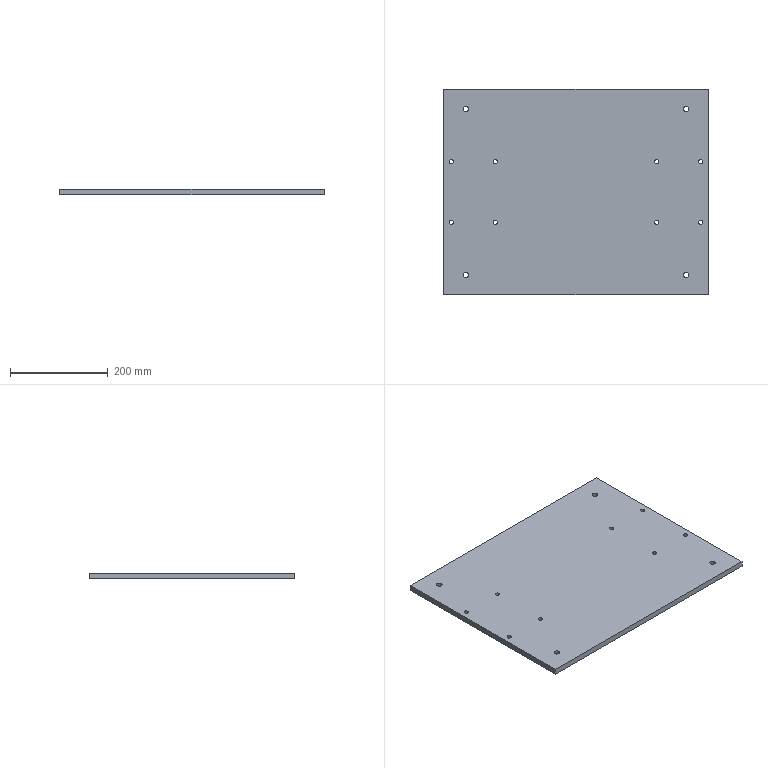Part | SolidWorks | features BaseBody 1 | 1 solid | 30 faces | box 540 x 420 x 12 mm | volume 2711591 mm3 | cylinder 24 | plane 6 | commonest cylinder face diameters 8.5 x16 11 x8
STEP:
#1=CARTESIAN_POINT('',(219.5,170.,-6.));
#2=VERTEX_POINT('',#1);
#3=CARTESIAN_POINT('',(230.5,170.,-6.));
#4=VERTEX_POINT('',#3);
#5=CARTESIAN_POINT('',(225.,170.,-6.));
#6=DIRECTION('',(0.,0.,1.));
#7=DIRECTION('',(1.,0.,0.));
#8=AXIS2_PLACEMENT_3D('',#5,#6,#7);
#9=CIRCLE('',#8,5.5);
#10=EDGE_CURVE('',#2,#4,#9,.T.);
#11=ORIENTED_EDGE('',*,*,#10,.F.);
#12=CARTESIAN_POINT('',(219.5,170.,6.));
#13=VERTEX_POINT('',#12);
#14=CARTESIAN_POINT('',(219.5,170.,-7.));
#15=DIRECTION('',(0.,0.,1.));
#16=VECTOR('',#15,1000.);
#17=LINE('',#14,#16);
#18=EDGE_CURVE('',#2,#13,#17,.T.);
#19=ORIENTED_EDGE('',*,*,#18,.T.);
#20=CARTESIAN_POINT('',(230.5,170.,6.));
#21=VERTEX_POINT('',#20);
#22=CARTESIAN_POINT('',(225.,170.,6.));
#23=DIRECTION('',(0.,0.,-1.));
#24=DIRECTION('',(1.,0.,0.));
#25=AXIS2_PLACEMENT_3D('',#22,#23,#24);
#26=CIRCLE('',#25,5.5);
#27=EDGE_CURVE('',#21,#13,#26,.T.);
#28=ORIENTED_EDGE('',*,*,#27,.F.);
#29=CARTESIAN_POINT('',(230.5,170.,-7.));
#30=DIRECTION('',(0.,0.,1.));
#31=VECTOR('',#30,1000.);
#32=LINE('',#29,#31);
#33=EDGE_CURVE('',#4,#21,#32,.T.);
#34=ORIENTED_EDGE('',*,*,#33,.F.);
#35=EDGE_LOOP('',(#11,#19,#28,#34));
#36=FACE_OUTER_BOUND('',#35,.T.);
#37=CARTESIAN_POINT('',(225.,170.,-7.));
#38=DIRECTION('',(0.,0.,1.));
#39=DIRECTION('',(1.,0.,0.));
#40=AXIS2_PLACEMENT_3D('',#37,#38,#39);
#41=CYLINDRICAL_SURFACE('',#40,5.5);
#42=ADVANCED_FACE('',(#36),#41,.F.);
#43=CARTESIAN_POINT('',(250.75,62.,-6.));
#44=VERTEX_POINT('',#43);
#45=CARTESIAN_POINT('',(259.25,62.,-6.));
#46=VERTEX_POINT('',#45);
#47=CARTESIAN_POINT('',(255.,62.,-6.));
#48=DIRECTION('',(0.,0.,1.));
#49=DIRECTION('',(1.,0.,0.));
#50=AXIS2_PLACEMENT_3D('',#47,#48,#49);
#51=CIRCLE('',#50,4.25);
#52=EDGE_CURVE('',#44,#46,#51,.T.);
#53=ORIENTED_EDGE('',*,*,#52,.F.);
#54=CARTESIAN_POINT('',(250.75,62.,6.));
#55=VERTEX_POINT('',#54);
#56=CARTESIAN_POINT('',(250.75,62.,-7.));
#57=DIRECTION('',(0.,0.,1.));
#58=VECTOR('',#57,1000.);
#59=LINE('',#56,#58);
#60=EDGE_CURVE('',#44,#55,#59,.T.);
#61=ORIENTED_EDGE('',*,*,#60,.T.);
#62=CARTESIAN_POINT('',(259.25,62.,6.));
#63=VERTEX_POINT('',#62);
#64=CARTESIAN_POINT('',(255.,62.,6.));
#65=DIRECTION('',(0.,0.,-1.));
#66=DIRECTION('',(1.,0.,0.));
#67=AXIS2_PLACEMENT_3D('',#64,#65,#66);
#68=CIRCLE('',#67,4.25);
#69=EDGE_CURVE('',#63,#55,#68,.T.);
#70=ORIENTED_EDGE('',*,*,#69,.F.);
#71=CARTESIAN_POINT('',(259.25,62.,-7.));
#72=DIRECTION('',(0.,0.,1.));
#73=VECTOR('',#72,1000.);
#74=LINE('',#71,#73);
#75=EDGE_CURVE('',#46,#63,#74,.T.);
#76=ORIENTED_EDGE('',*,*,#75,.F.);
#77=EDGE_LOOP('',(#53,#61,#70,#76));
#78=FACE_OUTER_BOUND('',#77,.T.);
#79=CARTESIAN_POINT('',(255.,62.,-7.));
#80=DIRECTION('',(0.,0.,1.));
#81=DIRECTION('',(1.,0.,0.));
#82=AXIS2_PLACEMENT_3D('',#79,#80,#81);
#83=CYLINDRICAL_SURFACE('',#82,4.25);
#84=ADVANCED_FACE('',(#78),#83,.F.);
#85=CARTESIAN_POINT('',(160.75,62.,-6.));
#86=VERTEX_POINT('',#85);
#87=CARTESIAN_POINT('',(169.25,62.,-6.));
#88=VERTEX_POINT('',#87);
#89=CARTESIAN_POINT('',(165.,62.,-6.));
#90=DIRECTION('',(0.,0.,1.));
#91=DIRECTION('',(1.,0.,0.));
#92=AXIS2_PLACEMENT_3D('',#89,#90,#91);
#93=CIRCLE('',#92,4.25);
#94=EDGE_CURVE('',#86,#88,#93,.T.);
#95=ORIENTED_EDGE('',*,*,#94,.F.);
#96=CARTESIAN_POINT('',(160.75,62.,6.));
#97=VERTEX_POINT('',#96);
#98=CARTESIAN_POINT('',(160.75,62.,-7.));
#99=DIRECTION('',(0.,0.,1.));
#100=VECTOR('',#99,1000.);
#101=LINE('',#98,#100);
#102=EDGE_CURVE('',#86,#97,#101,.T.);
#103=ORIENTED_EDGE('',*,*,#102,.T.);
#104=CARTESIAN_POINT('',(169.25,62.,6.));
#105=VERTEX_POINT('',#104);
#106=CARTESIAN_POINT('',(165.,62.,6.));
#107=DIRECTION('',(0.,0.,-1.));
#108=DIRECTION('',(1.,0.,0.));
#109=AXIS2_PLACEMENT_3D('',#106,#107,#108);
#110=CIRCLE('',#109,4.25);
#111=EDGE_CURVE('',#105,#97,#110,.T.);
#112=ORIENTED_EDGE('',*,*,#111,.F.);
#113=CARTESIAN_POINT('',(169.25,62.,-7.));
#114=DIRECTION('',(0.,0.,1.));
#115=VECTOR('',#114,1000.);
#116=LINE('',#113,#115);
#117=EDGE_CURVE('',#88,#105,#116,.T.);
#118=ORIENTED_EDGE('',*,*,#117,.F.);
#119=EDGE_LOOP('',(#95,#103,#112,#118));
#120=FACE_OUTER_BOUND('',#119,.T.);
#121=CARTESIAN_POINT('',(165.,62.,-7.));
#122=DIRECTION('',(0.,0.,1.));
#123=DIRECTION('',(1.,0.,0.));
#124=AXIS2_PLACEMENT_3D('',#121,#122,#123);
#125=CYLINDRICAL_SURFACE('',#124,4.25);
#126=ADVANCED_FACE('',(#120),#125,.F.);
#127=CARTESIAN_POINT('',(-230.5,170.,-6.));
#128=VERTEX_POINT('',#127);
#129=CARTESIAN_POINT('',(-219.5,170.,-6.));
#130=VERTEX_POINT('',#129);
#131=CARTESIAN_POINT('',(-225.,170.,-6.));
#132=DIRECTION('',(0.,0.,1.));
#133=DIRECTION('',(1.,0.,0.));
#134=AXIS2_PLACEMENT_3D('',#131,#132,#133);
#135=CIRCLE('',#134,5.5);
#136=EDGE_CURVE('',#128,#130,#135,.T.);
#137=ORIENTED_EDGE('',*,*,#136,.F.);
#138=CARTESIAN_POINT('',(-230.5,170.,6.));
#139=VERTEX_POINT('',#138);
#140=CARTESIAN_POINT('',(-230.5,170.,-7.));
#141=DIRECTION('',(0.,0.,1.));
#142=VECTOR('',#141,1000.);
#143=LINE('',#140,#142);
#144=EDGE_CURVE('',#128,#139,#143,.T.);
#145=ORIENTED_EDGE('',*,*,#144,.T.);
#146=CARTESIAN_POINT('',(-219.5,170.,6.));
#147=VERTEX_POINT('',#146);
#148=CARTESIAN_POINT('',(-225.,170.,6.));
#149=DIRECTION('',(0.,0.,-1.));
#150=DIRECTION('',(1.,0.,0.));
#151=AXIS2_PLACEMENT_3D('',#148,#149,#150);
#152=CIRCLE('',#151,5.5);
#153=EDGE_CURVE('',#147,#139,#152,.T.);
#154=ORIENTED_EDGE('',*,*,#153,.F.);
#155=CARTESIAN_POINT('',(-219.5,170.,-7.));
#156=DIRECTION('',(0.,0.,1.));
#157=VECTOR('',#156,1000.);
#158=LINE('',#155,#157);
#159=EDGE_CURVE('',#130,#147,#158,.T.);
#160=ORIENTED_EDGE('',*,*,#159,.F.);
#161=EDGE_LOOP('',(#137,#145,#154,#160));
#162=FACE_OUTER_BOUND('',#161,.T.);
#163=CARTESIAN_POINT('',(-225.,170.,-7.));
#164=DIRECTION('',(0.,0.,1.));
#165=DIRECTION('',(1.,0.,0.));
#166=AXIS2_PLACEMENT_3D('',#163,#164,#165);
#167=CYLINDRICAL_SURFACE('',#166,5.5);
#168=ADVANCED_FACE('',(#162),#167,.F.);
#169=CARTESIAN_POINT('',(-169.25,62.,-6.));
#170=VERTEX_POINT('',#169);
#171=CARTESIAN_POINT('',(-160.75,62.,-6.));
#172=VERTEX_POINT('',#171);
#173=CARTESIAN_POINT('',(-165.,62.,-6.));
#174=DIRECTION('',(0.,0.,1.));
#175=DIRECTION('',(1.,0.,0.));
#176=AXIS2_PLACEMENT_3D('',#173,#174,#175);
#177=CIRCLE('',#176,4.25);
#178=EDGE_CURVE('',#170,#172,#177,.T.);
#179=ORIENTED_EDGE('',*,*,#178,.F.);
#180=CARTESIAN_POINT('',(-169.25,62.,6.));
#181=VERTEX_POINT('',#180);
#182=CARTESIAN_POINT('',(-169.25,62.,-7.));
#183=DIRECTION('',(0.,0.,1.));
#184=VECTOR('',#183,1000.);
#185=LINE('',#182,#184);
#186=EDGE_CURVE('',#170,#181,#185,.T.);
#187=ORIENTED_EDGE('',*,*,#186,.T.);
#188=CARTESIAN_POINT('',(-160.75,62.,6.));
#189=VERTEX_POINT('',#188);
#190=CARTESIAN_POINT('',(-165.,62.,6.));
#191=DIRECTION('',(0.,0.,-1.));
#192=DIRECTION('',(1.,0.,0.));
#193=AXIS2_PLACEMENT_3D('',#190,#191,#192);
#194=CIRCLE('',#193,4.25);
#195=EDGE_CURVE('',#189,#181,#194,.T.);
#196=ORIENTED_EDGE('',*,*,#195,.F.);
#197=CARTESIAN_POINT('',(-160.75,62.,-7.));
#198=DIRECTION('',(0.,0.,1.));
#199=VECTOR('',#198,1000.);
#200=LINE('',#197,#199);
#201=EDGE_CURVE('',#172,#189,#200,.T.);
#202=ORIENTED_EDGE('',*,*,#201,.F.);
#203=EDGE_LOOP('',(#179,#187,#196,#202));
#204=FACE_OUTER_BOUND('',#203,.T.);
#205=CARTESIAN_POINT('',(-165.,62.,-7.));
#206=DIRECTION('',(0.,0.,1.));
#207=DIRECTION('',(1.,0.,0.));
#208=AXIS2_PLACEMENT_3D('',#205,#206,#207);
#209=CYLINDRICAL_SURFACE('',#208,4.25);
#210=ADVANCED_FACE('',(#204),#209,.F.);
#211=CARTESIAN_POINT('',(-259.25,62.,-6.));
#212=VERTEX_POINT('',#211);
#213=CARTESIAN_POINT('',(-250.75,62.,-6.));
#214=VERTEX_POINT('',#213);
#215=CARTESIAN_POINT('',(-255.,62.,-6.));
#216=DIRECTION('',(0.,0.,1.));
#217=DIRECTION('',(1.,0.,0.));
#218=AXIS2_PLACEMENT_3D('',#215,#216,#217);
#219=CIRCLE('',#218,4.25);
#220=EDGE_CURVE('',#212,#214,#219,.T.);
#221=ORIENTED_EDGE('',*,*,#220,.F.);
#222=CARTESIAN_POINT('',(-259.25,62.,6.));
#223=VERTEX_POINT('',#222);
#224=CARTESIAN_POINT('',(-259.25,62.,-7.));
#225=DIRECTION('',(0.,0.,1.));
#226=VECTOR('',#225,1000.);
#227=LINE('',#224,#226);
#228=EDGE_CURVE('',#212,#223,#227,.T.);
#229=ORIENTED_EDGE('',*,*,#228,.T.);
#230=CARTESIAN_POINT('',(-250.75,62.,6.));
#231=VERTEX_POINT('',#230);
#232=CARTESIAN_POINT('',(-255.,62.,6.));
#233=DIRECTION('',(0.,0.,-1.));
#234=DIRECTION('',(1.,0.,0.));
#235=AXIS2_PLACEMENT_3D('',#232,#233,#234);
#236=CIRCLE('',#235,4.25);
#237=EDGE_CURVE('',#231,#223,#236,.T.);
#238=ORIENTED_EDGE('',*,*,#237,.F.);
#239=CARTESIAN_POINT('',(-250.75,62.,-7.));
#240=DIRECTION('',(0.,0.,1.));
#241=VECTOR('',#240,1000.);
#242=LINE('',#239,#241);
#243=EDGE_CURVE('',#214,#231,#242,.T.);
#244=ORIENTED_EDGE('',*,*,#243,.F.);
#245=EDGE_LOOP('',(#221,#229,#238,#244));
#246=FACE_OUTER_BOUND('',#245,.T.);
#247=CARTESIAN_POINT('',(-255.,62.,-7.));
#248=DIRECTION('',(0.,0.,1.));
#249=DIRECTION('',(1.,0.,0.));
#250=AXIS2_PLACEMENT_3D('',#247,#248,#249);
#251=CYLINDRICAL_SURFACE('',#250,4.25);
#252=ADVANCED_FACE('',(#246),#251,.F.);
#253=CARTESIAN_POINT('',(250.75,-62.,-6.));
#254=VERTEX_POINT('',#253);
#255=CARTESIAN_POINT('',(259.25,-62.,-6.));
#256=VERTEX_POINT('',#255);
#257=CARTESIAN_POINT('',(255.,-62.,-6.));
#258=DIRECTION('',(0.,0.,1.));
#259=DIRECTION('',(1.,0.,0.));
#260=AXIS2_PLACEMENT_3D('',#257,#258,#259);
#261=CIRCLE('',#260,4.25);
#262=EDGE_CURVE('',#254,#256,#261,.T.);
#263=ORIENTED_EDGE('',*,*,#262,.F.);
#264=CARTESIAN_POINT('',(250.75,-62.,6.));
#265=VERTEX_POINT('',#264);
#266=CARTESIAN_POINT('',(250.75,-62.,-7.));
#267=DIRECTION('',(0.,0.,1.));
#268=VECTOR('',#267,1000.);
#269=LINE('',#266,#268);
#270=EDGE_CURVE('',#254,#265,#269,.T.);
#271=ORIENTED_EDGE('',*,*,#270,.T.);
#272=CARTESIAN_POINT('',(259.25,-62.,6.));
#273=VERTEX_POINT('',#272);
#274=CARTESIAN_POINT('',(255.,-62.,6.));
#275=DIRECTION('',(0.,0.,-1.));
#276=DIRECTION('',(1.,0.,0.));
#277=AXIS2_PLACEMENT_3D('',#274,#275,#276);
#278=CIRCLE('',#277,4.25);
#279=EDGE_CURVE('',#273,#265,#278,.T.);
#280=ORIENTED_EDGE('',*,*,#279,.F.);
#281=CARTESIAN_POINT('',(259.25,-62.,-7.));
#282=DIRECTION('',(0.,0.,1.));
#283=VECTOR('',#282,1000.);
#284=LINE('',#281,#283);
#285=EDGE_CURVE('',#256,#273,#284,.T.);
#286=ORIENTED_EDGE('',*,*,#285,.F.);
#287=EDGE_LOOP('',(#263,#271,#280,#286));
#288=FACE_OUTER_BOUND('',#287,.T.);
#289=CARTESIAN_POINT('',(255.,-62.,-7.));
#290=DIRECTION('',(0.,0.,1.));
#291=DIRECTION('',(1.,0.,0.));
#292=AXIS2_PLACEMENT_3D('',#289,#290,#291);
#293=CYLINDRICAL_SURFACE('',#292,4.25);
#294=ADVANCED_FACE('',(#288),#293,.F.);
#295=CARTESIAN_POINT('',(160.75,-62.,-6.));
#296=VERTEX_POINT('',#295);
#297=CARTESIAN_POINT('',(169.25,-62.,-6.));
#298=VERTEX_POINT('',#297);
#299=CARTESIAN_POINT('',(165.,-62.,-6.));
#300=DIRECTION('',(0.,0.,1.));
#301=DIRECTION('',(1.,0.,0.));
#302=AXIS2_PLACEMENT_3D('',#299,#300,#301);
#303=CIRCLE('',#302,4.25);
#304=EDGE_CURVE('',#296,#298,#303,.T.);
#305=ORIENTED_EDGE('',*,*,#304,.F.);
#306=CARTESIAN_POINT('',(160.75,-62.,6.));
#307=VERTEX_POINT('',#306);
#308=CARTESIAN_POINT('',(160.75,-62.,-7.));
#309=DIRECTION('',(0.,0.,1.));
#310=VECTOR('',#309,1000.);
#311=LINE('',#308,#310);
#312=EDGE_CURVE('',#296,#307,#311,.T.);
#313=ORIENTED_EDGE('',*,*,#312,.T.);
#314=CARTESIAN_POINT('',(169.25,-62.,6.));
#315=VERTEX_POINT('',#314);
#316=CARTESIAN_POINT('',(165.,-62.,6.));
#317=DIRECTION('',(0.,0.,-1.));
#318=DIRECTION('',(1.,0.,0.));
#319=AXIS2_PLACEMENT_3D('',#316,#317,#318);
#320=CIRCLE('',#319,4.25);
#321=EDGE_CURVE('',#315,#307,#320,.T.);
#322=ORIENTED_EDGE('',*,*,#321,.F.);
#323=CARTESIAN_POINT('',(169.25,-62.,-7.));
#324=DIRECTION('',(0.,0.,1.));
#325=VECTOR('',#324,1000.);
#326=LINE('',#323,#325);
#327=EDGE_CURVE('',#298,#315,#326,.T.);
#328=ORIENTED_EDGE('',*,*,#327,.F.);
#329=EDGE_LOOP('',(#305,#313,#322,#328));
#330=FACE_OUTER_BOUND('',#329,.T.);
#331=CARTESIAN_POINT('',(165.,-62.,-7.));
#332=DIRECTION('',(0.,0.,1.));
#333=DIRECTION('',(1.,0.,0.));
#334=AXIS2_PLACEMENT_3D('',#331,#332,#333);
#335=CYLINDRICAL_SURFACE('',#334,4.25);
#336=ADVANCED_FACE('',(#330),#335,.F.);
#337=CARTESIAN_POINT('',(219.5,-170.,-6.));
#338=VERTEX_POINT('',#337);
#339=CARTESIAN_POINT('',(230.5,-170.,-6.));
#340=VERTEX_POINT('',#339);
#341=CARTESIAN_POINT('',(225.,-170.,-6.));
#342=DIRECTION('',(0.,0.,1.));
#343=DIRECTION('',(1.,0.,0.));
#344=AXIS2_PLACEMENT_3D('',#341,#342,#343);
#345=CIRCLE('',#344,5.5);
#346=EDGE_CURVE('',#338,#340,#345,.T.);
#347=ORIENTED_EDGE('',*,*,#346,.F.);
#348=CARTESIAN_POINT('',(219.5,-170.,6.));
#349=VERTEX_POINT('',#348);
#350=CARTESIAN_POINT('',(219.5,-170.,-7.));
#351=DIRECTION('',(0.,0.,1.));
#352=VECTOR('',#351,1000.);
#353=LINE('',#350,#352);
#354=EDGE_CURVE('',#338,#349,#353,.T.);
#355=ORIENTED_EDGE('',*,*,#354,.T.);
#356=CARTESIAN_POINT('',(230.5,-170.,6.));
#357=VERTEX_POINT('',#356);
#358=CARTESIAN_POINT('',(225.,-170.,6.));
#359=DIRECTION('',(0.,0.,-1.));
#360=DIRECTION('',(1.,0.,0.));
#361=AXIS2_PLACEMENT_3D('',#358,#359,#360);
#362=CIRCLE('',#361,5.5);
#363=EDGE_CURVE('',#357,#349,#362,.T.);
#364=ORIENTED_EDGE('',*,*,#363,.F.);
#365=CARTESIAN_POINT('',(230.5,-170.,-7.));
#366=DIRECTION('',(0.,0.,1.));
#367=VECTOR('',#366,1000.);
#368=LINE('',#365,#367);
#369=EDGE_CURVE('',#340,#357,#368,.T.);
#370=ORIENTED_EDGE('',*,*,#369,.F.);
#371=EDGE_LOOP('',(#347,#355,#364,#370));
#372=FACE_OUTER_BOUND('',#371,.T.);
#373=CARTESIAN_POINT('',(225.,-170.,-7.));
#374=DIRECTION('',(0.,0.,1.));
#375=DIRECTION('',(1.,0.,0.));
#376=AXIS2_PLACEMENT_3D('',#373,#374,#375);
#377=CYLINDRICAL_SURFACE('',#376,5.5);
#378=ADVANCED_FACE('',(#372),#377,.F.);
#379=CARTESIAN_POINT('',(-169.25,-62.,-6.));
#380=VERTEX_POINT('',#379);
#381=CARTESIAN_POINT('',(-160.75,-62.,-6.));
#382=VERTEX_POINT('',#381);
#383=CARTESIAN_POINT('',(-165.,-62.,-6.));
#384=DIRECTION('',(0.,0.,1.));
#385=DIRECTION('',(1.,0.,0.));
#386=AXIS2_PLACEMENT_3D('',#383,#384,#385);
#387=CIRCLE('',#386,4.25);
#388=EDGE_CURVE('',#380,#382,#387,.T.);
#389=ORIENTED_EDGE('',*,*,#388,.F.);
#390=CARTESIAN_POINT('',(-169.25,-62.,6.));
#391=VERTEX_POINT('',#390);
#392=CARTESIAN_POINT('',(-169.25,-62.,-7.));
#393=DIRECTION('',(0.,0.,1.));
#394=VECTOR('',#393,1000.);
#395=LINE('',#392,#394);
#396=EDGE_CURVE('',#380,#391,#395,.T.);
#397=ORIENTED_EDGE('',*,*,#396,.T.);
#398=CARTESIAN_POINT('',(-160.75,-62.,6.));
#399=VERTEX_POINT('',#398);
#400=CARTESIAN_POINT('',(-165.,-62.,6.));
#401=DIRECTION('',(0.,0.,-1.));
#402=DIRECTION('',(1.,0.,0.));
#403=AXIS2_PLACEMENT_3D('',#400,#401,#402);
#404=CIRCLE('',#403,4.25);
#405=EDGE_CURVE('',#399,#391,#404,.T.);
#406=ORIENTED_EDGE('',*,*,#405,.F.);
#407=CARTESIAN_POINT('',(-160.75,-62.,-7.));
#408=DIRECTION('',(0.,0.,1.));
#409=VECTOR('',#408,1000.);
#410=LINE('',#407,#409);
#411=EDGE_CURVE('',#382,#399,#410,.T.);
#412=ORIENTED_EDGE('',*,*,#411,.F.);
#413=EDGE_LOOP('',(#389,#397,#406,#412));
#414=FACE_OUTER_BOUND('',#413,.T.);
#415=CARTESIAN_POINT('',(-165.,-62.,-7.));
#416=DIRECTION('',(0.,0.,1.));
#417=DIRECTION('',(1.,0.,0.));
#418=AXIS2_PLACEMENT_3D('',#415,#416,#417);
#419=CYLINDRICAL_SURFACE('',#418,4.25);
#420=ADVANCED_FACE('',(#414),#419,.F.);
#421=CARTESIAN_POINT('',(-259.25,-62.,-6.));
#422=VERTEX_POINT('',#421);
#423=CARTESIAN_POINT('',(-250.75,-62.,-6.));
#424=VERTEX_POINT('',#423);
#425=CARTESIAN_POINT('',(-255.,-62.,-6.));
#426=DIRECTION('',(0.,0.,1.));
#427=DIRECTION('',(1.,0.,0.));
#428=AXIS2_PLACEMENT_3D('',#425,#426,#427);
#429=CIRCLE('',#428,4.25);
#430=EDGE_CURVE('',#422,#424,#429,.T.);
#431=ORIENTED_EDGE('',*,*,#430,.F.);
#432=CARTESIAN_POINT('',(-259.25,-62.,6.));
#433=VERTEX_POINT('',#432);
#434=CARTESIAN_POINT('',(-259.25,-62.,-7.));
#435=DIRECTION('',(0.,0.,1.));
#436=VECTOR('',#435,1000.);
#437=LINE('',#434,#436);
#438=EDGE_CURVE('',#422,#433,#437,.T.);
#439=ORIENTED_EDGE('',*,*,#438,.T.);
#440=CARTESIAN_POINT('',(-250.75,-62.,6.));
#441=VERTEX_POINT('',#440);
#442=CARTESIAN_POINT('',(-255.,-62.,6.));
#443=DIRECTION('',(0.,0.,-1.));
#444=DIRECTION('',(1.,0.,0.));
#445=AXIS2_PLACEMENT_3D('',#442,#443,#444);
#446=CIRCLE('',#445,4.25);
#447=EDGE_CURVE('',#441,#433,#446,.T.);
#448=ORIENTED_EDGE('',*,*,#447,.F.);
#449=CARTESIAN_POINT('',(-250.75,-62.,-7.));
#450=DIRECTION('',(0.,0.,1.));
#451=VECTOR('',#450,1000.);
#452=LINE('',#449,#451);
#453=EDGE_CURVE('',#424,#441,#452,.T.);
#454=ORIENTED_EDGE('',*,*,#453,.F.);
#455=EDGE_LOOP('',(#431,#439,#448,#454));
#456=FACE_OUTER_BOUND('',#455,.T.);
#457=CARTESIAN_POINT('',(-255.,-62.,-7.));
#458=DIRECTION('',(0.,0.,1.));
#459=DIRECTION('',(1.,0.,0.));
#460=AXIS2_PLACEMENT_3D('',#457,#458,#459);
#461=CYLINDRICAL_SURFACE('',#460,4.25);
#462=ADVANCED_FACE('',(#456),#461,.F.);
#463=CARTESIAN_POINT('',(-230.5,-170.,-6.));
#464=VERTEX_POINT('',#463);
#465=CARTESIAN_POINT('',(-219.5,-170.,-6.));
#466=VERTEX_POINT('',#465);
#467=CARTESIAN_POINT('',(-225.,-170.,-6.));
#468=DIRECTION('',(0.,0.,1.));
#469=DIRECTION('',(1.,0.,0.));
#470=AXIS2_PLACEMENT_3D('',#467,#468,#469);
#471=CIRCLE('',#470,5.5);
#472=EDGE_CURVE('',#464,#466,#471,.T.);
#473=ORIENTED_EDGE('',*,*,#472,.F.);
#474=CARTESIAN_POINT('',(-230.5,-170.,6.));
#475=VERTEX_POINT('',#474);
#476=CARTESIAN_POINT('',(-230.5,-170.,-7.));
#477=DIRECTION('',(0.,0.,1.));
#478=VECTOR('',#477,1000.);
#479=LINE('',#476,#478);
#480=EDGE_CURVE('',#464,#475,#479,.T.);
#481=ORIENTED_EDGE('',*,*,#480,.T.);
#482=CARTESIAN_POINT('',(-219.5,-170.,6.));
#483=VERTEX_POINT('',#482);
#484=CARTESIAN_POINT('',(-225.,-170.,6.));
#485=DIRECTION('',(0.,0.,-1.));
#486=DIRECTION('',(1.,0.,0.));
#487=AXIS2_PLACEMENT_3D('',#484,#485,#486);
#488=CIRCLE('',#487,5.5);
#489=EDGE_CURVE('',#483,#475,#488,.T.);
#490=ORIENTED_EDGE('',*,*,#489,.F.);
#491=CARTESIAN_POINT('',(-219.5,-170.,-7.));
#492=DIRECTION('',(0.,0.,1.));
#493=VECTOR('',#492,1000.);
#494=LINE('',#491,#493);
#495=EDGE_CURVE('',#466,#483,#494,.T.);
#496=ORIENTED_EDGE('',*,*,#495,.F.);
#497=EDGE_LOOP('',(#473,#481,#490,#496));
#498=FACE_OUTER_BOUND('',#497,.T.);
#499=CARTESIAN_POINT('',(-225.,-170.,-7.));
#500=DIRECTION('',(0.,0.,1.));
#501=DIRECTION('',(1.,0.,0.));
#502=AXIS2_PLACEMENT_3D('',#499,#500,#501);
#503=CYLINDRICAL_SURFACE('',#502,5.5);
#504=ADVANCED_FACE('',(#498),#503,.F.);
#505=ORIENTED_EDGE('',*,*,#27,.T.);
#506=CARTESIAN_POINT('',(225.,170.,6.));
#507=DIRECTION('',(0.,0.,-1.));
#508=DIRECTION('',(1.,0.,0.));
#509=AXIS2_PLACEMENT_3D('',#506,#507,#508);
#510=CIRCLE('',#509,5.5);
#511=EDGE_CURVE('',#13,#21,#510,.T.);
#512=ORIENTED_EDGE('',*,*,#511,.T.);
#513=EDGE_LOOP('',(#505,#512));
#514=FACE_BOUND('',#513,.T.);
#515=ORIENTED_EDGE('',*,*,#69,.T.);
#516=CARTESIAN_POINT('',(255.,62.,6.));
#517=DIRECTION('',(0.,0.,-1.));
#518=DIRECTION('',(1.,0.,0.));
#519=AXIS2_PLACEMENT_3D('',#516,#517,#518);
#520=CIRCLE('',#519,4.25);
#521=EDGE_CURVE('',#55,#63,#520,.T.);
#522=ORIENTED_EDGE('',*,*,#521,.T.);
#523=EDGE_LOOP('',(#515,#522));
#524=FACE_BOUND('',#523,.T.);
#525=ORIENTED_EDGE('',*,*,#111,.T.);
#526=CARTESIAN_POINT('',(165.,62.,6.));
#527=DIRECTION('',(0.,0.,-1.));
#528=DIRECTION('',(1.,0.,0.));
#529=AXIS2_PLACEMENT_3D('',#526,#527,#528);
#530=CIRCLE('',#529,4.25);
#531=EDGE_CURVE('',#97,#105,#530,.T.);
#532=ORIENTED_EDGE('',*,*,#531,.T.);
#533=EDGE_LOOP('',(#525,#532));
#534=FACE_BOUND('',#533,.T.);
#535=ORIENTED_EDGE('',*,*,#153,.T.);
#536=CARTESIAN_POINT('',(-225.,170.,6.));
#537=DIRECTION('',(0.,0.,-1.));
#538=DIRECTION('',(1.,0.,0.));
#539=AXIS2_PLACEMENT_3D('',#536,#537,#538);
#540=CIRCLE('',#539,5.5);
#541=EDGE_CURVE('',#139,#147,#540,.T.);
#542=ORIENTED_EDGE('',*,*,#541,.T.);
#543=EDGE_LOOP('',(#535,#542));
#544=FACE_BOUND('',#543,.T.);
#545=ORIENTED_EDGE('',*,*,#195,.T.);
#546=CARTESIAN_POINT('',(-165.,62.,6.));
#547=DIRECTION('',(0.,0.,-1.));
#548=DIRECTION('',(1.,0.,0.));
#549=AXIS2_PLACEMENT_3D('',#546,#547,#548);
#550=CIRCLE('',#549,4.25);
#551=EDGE_CURVE('',#181,#189,#550,.T.);
#552=ORIENTED_EDGE('',*,*,#551,.T.);
#553=EDGE_LOOP('',(#545,#552));
#554=FACE_BOUND('',#553,.T.);
#555=ORIENTED_EDGE('',*,*,#237,.T.);
#556=CARTESIAN_POINT('',(-255.,62.,6.));
#557=DIRECTION('',(0.,0.,-1.));
#558=DIRECTION('',(1.,0.,0.));
#559=AXIS2_PLACEMENT_3D('',#556,#557,#558);
#560=CIRCLE('',#559,4.25);
#561=EDGE_CURVE('',#223,#231,#560,.T.);
#562=ORIENTED_EDGE('',*,*,#561,.T.);
#563=EDGE_LOOP('',(#555,#562));
#564=FACE_BOUND('',#563,.T.);
#565=ORIENTED_EDGE('',*,*,#279,.T.);
#566=CARTESIAN_POINT('',(255.,-62.,6.));
#567=DIRECTION('',(0.,0.,-1.));
#568=DIRECTION('',(1.,0.,0.));
#569=AXIS2_PLACEMENT_3D('',#566,#567,#568);
#570=CIRCLE('',#569,4.25);
#571=EDGE_CURVE('',#265,#273,#570,.T.);
#572=ORIENTED_EDGE('',*,*,#571,.T.);
#573=EDGE_LOOP('',(#565,#572));
#574=FACE_BOUND('',#573,.T.);
#575=ORIENTED_EDGE('',*,*,#321,.T.);
#576=CARTESIAN_POINT('',(165.,-62.,6.));
#577=DIRECTION('',(0.,0.,-1.));
#578=DIRECTION('',(1.,0.,0.));
#579=AXIS2_PLACEMENT_3D('',#576,#577,#578);
#580=CIRCLE('',#579,4.25);
#581=EDGE_CURVE('',#307,#315,#580,.T.);
#582=ORIENTED_EDGE('',*,*,#581,.T.);
#583=EDGE_LOOP('',(#575,#582));
#584=FACE_BOUND('',#583,.T.);
#585=ORIENTED_EDGE('',*,*,#363,.T.);
#586=CARTESIAN_POINT('',(225.,-170.,6.));
#587=DIRECTION('',(0.,0.,-1.));
#588=DIRECTION('',(1.,0.,0.));
#589=AXIS2_PLACEMENT_3D('',#586,#587,#588);
#590=CIRCLE('',#589,5.5);
#591=EDGE_CURVE('',#349,#357,#590,.T.);
#592=ORIENTED_EDGE('',*,*,#591,.T.);
#593=EDGE_LOOP('',(#585,#592));
#594=FACE_BOUND('',#593,.T.);
#595=ORIENTED_EDGE('',*,*,#405,.T.);
#596=CARTESIAN_POINT('',(-165.,-62.,6.));
#597=DIRECTION('',(0.,0.,-1.));
#598=DIRECTION('',(1.,0.,0.));
#599=AXIS2_PLACEMENT_3D('',#596,#597,#598);
#600=CIRCLE('',#599,4.25);
#601=EDGE_CURVE('',#391,#399,#600,.T.);
#602=ORIENTED_EDGE('',*,*,#601,.T.);
#603=EDGE_LOOP('',(#595,#602));
#604=FACE_BOUND('',#603,.T.);
#605=ORIENTED_EDGE('',*,*,#447,.T.);
#606=CARTESIAN_POINT('',(-255.,-62.,6.));
#607=DIRECTION('',(0.,0.,-1.));
#608=DIRECTION('',(1.,0.,0.));
#609=AXIS2_PLACEMENT_3D('',#606,#607,#608);
#610=CIRCLE('',#609,4.25);
#611=EDGE_CURVE('',#433,#441,#610,.T.);
#612=ORIENTED_EDGE('',*,*,#611,.T.);
#613=EDGE_LOOP('',(#605,#612));
#614=FACE_BOUND('',#613,.T.);
#615=ORIENTED_EDGE('',*,*,#489,.T.);
#616=CARTESIAN_POINT('',(-225.,-170.,6.));
#617=DIRECTION('',(0.,0.,-1.));
#618=DIRECTION('',(1.,0.,0.));
#619=AXIS2_PLACEMENT_3D('',#616,#617,#618);
#620=CIRCLE('',#619,5.5);
#621=EDGE_CURVE('',#475,#483,#620,.T.);
#622=ORIENTED_EDGE('',*,*,#621,.T.);
#623=EDGE_LOOP('',(#615,#622));
#624=FACE_BOUND('',#623,.T.);
#625=CARTESIAN_POINT('',(270.,-210.,6.));
#626=VERTEX_POINT('',#625);
#627=CARTESIAN_POINT('',(270.,210.,6.));
#628=VERTEX_POINT('',#627);
#629=CARTESIAN_POINT('',(270.,-210.,6.));
#630=DIRECTION('',(0.,1.,0.));
#631=VECTOR('',#630,1000.);
#632=LINE('',#629,#631);
#633=EDGE_CURVE('',#626,#628,#632,.T.);
#634=ORIENTED_EDGE('',*,*,#633,.T.);
#635=CARTESIAN_POINT('',(-270.,210.,6.));
#636=VERTEX_POINT('',#635);
#637=CARTESIAN_POINT('',(-270.,210.,6.));
#638=DIRECTION('',(-1.,0.,0.));
#639=VECTOR('',#638,1000.);
#640=LINE('',#637,#639);
#641=EDGE_CURVE('',#628,#636,#640,.T.);
#642=ORIENTED_EDGE('',*,*,#641,.T.);
#643=CARTESIAN_POINT('',(-270.,-210.,6.));
#644=VERTEX_POINT('',#643);
#645=CARTESIAN_POINT('',(-270.,-210.,6.));
#646=DIRECTION('',(0.,-1.,0.));
#647=VECTOR('',#646,1000.);
#648=LINE('',#645,#647);
#649=EDGE_CURVE('',#636,#644,#648,.T.);
#650=ORIENTED_EDGE('',*,*,#649,.T.);
#651=CARTESIAN_POINT('',(-270.,-210.,6.));
#652=DIRECTION('',(1.,0.,0.));
#653=VECTOR('',#652,1000.);
#654=LINE('',#651,#653);
#655=EDGE_CURVE('',#644,#626,#654,.T.);
#656=ORIENTED_EDGE('',*,*,#655,.T.);
#657=EDGE_LOOP('',(#634,#642,#650,#656));
#658=FACE_OUTER_BOUND('',#657,.T.);
#659=CARTESIAN_POINT('',(-270.,-210.,6.));
#660=DIRECTION('',(0.,0.,1.));
#661=DIRECTION('',(1.,0.,0.));
#662=AXIS2_PLACEMENT_3D('',#659,#660,#661);
#663=PLANE('',#662);
#664=ADVANCED_FACE('',(#514,#524,#534,#544,#554,#564,#574,#584,#594,#604,#614,#624,#658),#663,.T.);
#665=ORIENTED_EDGE('',*,*,#18,.F.);
#666=CARTESIAN_POINT('',(225.,170.,-6.));
#667=DIRECTION('',(0.,0.,1.));
#668=DIRECTION('',(1.,0.,0.));
#669=AXIS2_PLACEMENT_3D('',#666,#667,#668);
#670=CIRCLE('',#669,5.5);
#671=EDGE_CURVE('',#4,#2,#670,.T.);
#672=ORIENTED_EDGE('',*,*,#671,.F.);
#673=ORIENTED_EDGE('',*,*,#33,.T.);
#674=ORIENTED_EDGE('',*,*,#511,.F.);
#675=EDGE_LOOP('',(#665,#672,#673,#674));
#676=FACE_OUTER_BOUND('',#675,.T.);
#677=CARTESIAN_POINT('',(225.,170.,-7.));
#678=DIRECTION('',(0.,0.,1.));
#679=DIRECTION('',(1.,0.,0.));
#680=AXIS2_PLACEMENT_3D('',#677,#678,#679);
#681=CYLINDRICAL_SURFACE('',#680,5.5);
#682=ADVANCED_FACE('',(#676),#681,.F.);
#683=ORIENTED_EDGE('',*,*,#60,.F.);
#684=CARTESIAN_POINT('',(255.,62.,-6.));
#685=DIRECTION('',(0.,0.,1.));
#686=DIRECTION('',(1.,0.,0.));
#687=AXIS2_PLACEMENT_3D('',#684,#685,#686);
#688=CIRCLE('',#687,4.25);
#689=EDGE_CURVE('',#46,#44,#688,.T.);
#690=ORIENTED_EDGE('',*,*,#689,.F.);
#691=ORIENTED_EDGE('',*,*,#75,.T.);
#692=ORIENTED_EDGE('',*,*,#521,.F.);
#693=EDGE_LOOP('',(#683,#690,#691,#692));
#694=FACE_OUTER_BOUND('',#693,.T.);
#695=CARTESIAN_POINT('',(255.,62.,-7.));
#696=DIRECTION('',(0.,0.,1.));
#697=DIRECTION('',(1.,0.,0.));
#698=AXIS2_PLACEMENT_3D('',#695,#696,#697);
#699=CYLINDRICAL_SURFACE('',#698,4.25);
#700=ADVANCED_FACE('',(#694),#699,.F.);
#701=ORIENTED_EDGE('',*,*,#102,.F.);
#702=CARTESIAN_POINT('',(165.,62.,-6.));
#703=DIRECTION('',(0.,0.,1.));
#704=DIRECTION('',(1.,0.,0.));
#705=AXIS2_PLACEMENT_3D('',#702,#703,#704);
#706=CIRCLE('',#705,4.25);
#707=EDGE_CURVE('',#88,#86,#706,.T.);
#708=ORIENTED_EDGE('',*,*,#707,.F.);
#709=ORIENTED_EDGE('',*,*,#117,.T.);
#710=ORIENTED_EDGE('',*,*,#531,.F.);
#711=EDGE_LOOP('',(#701,#708,#709,#710));
#712=FACE_OUTER_BOUND('',#711,.T.);
#713=CARTESIAN_POINT('',(165.,62.,-7.));
#714=DIRECTION('',(0.,0.,1.));
#715=DIRECTION('',(1.,0.,0.));
#716=AXIS2_PLACEMENT_3D('',#713,#714,#715);
#717=CYLINDRICAL_SURFACE('',#716,4.25);
#718=ADVANCED_FACE('',(#712),#717,.F.);
#719=ORIENTED_EDGE('',*,*,#144,.F.);
#720=CARTESIAN_POINT('',(-225.,170.,-6.));
#721=DIRECTION('',(0.,0.,1.));
#722=DIRECTION('',(1.,0.,0.));
#723=AXIS2_PLACEMENT_3D('',#720,#721,#722);
#724=CIRCLE('',#723,5.5);
#725=EDGE_CURVE('',#130,#128,#724,.T.);
#726=ORIENTED_EDGE('',*,*,#725,.F.);
#727=ORIENTED_EDGE('',*,*,#159,.T.);
#728=ORIENTED_EDGE('',*,*,#541,.F.);
#729=EDGE_LOOP('',(#719,#726,#727,#728));
#730=FACE_OUTER_BOUND('',#729,.T.);
#731=CARTESIAN_POINT('',(-225.,170.,-7.));
#732=DIRECTION('',(0.,0.,1.));
#733=DIRECTION('',(1.,0.,0.));
#734=AXIS2_PLACEMENT_3D('',#731,#732,#733);
#735=CYLINDRICAL_SURFACE('',#734,5.5);
#736=ADVANCED_FACE('',(#730),#735,.F.);
#737=ORIENTED_EDGE('',*,*,#186,.F.);
#738=CARTESIAN_POINT('',(-165.,62.,-6.));
#739=DIRECTION('',(0.,0.,1.));
#740=DIRECTION('',(1.,0.,0.));
#741=AXIS2_PLACEMENT_3D('',#738,#739,#740);
#742=CIRCLE('',#741,4.25);
#743=EDGE_CURVE('',#172,#170,#742,.T.);
#744=ORIENTED_EDGE('',*,*,#743,.F.);
#745=ORIENTED_EDGE('',*,*,#201,.T.);
#746=ORIENTED_EDGE('',*,*,#551,.F.);
#747=EDGE_LOOP('',(#737,#744,#745,#746));
#748=FACE_OUTER_BOUND('',#747,.T.);
#749=CARTESIAN_POINT('',(-165.,62.,-7.));
#750=DIRECTION('',(0.,0.,1.));
#751=DIRECTION('',(1.,0.,0.));
#752=AXIS2_PLACEMENT_3D('',#749,#750,#751);
#753=CYLINDRICAL_SURFACE('',#752,4.25);
#754=ADVANCED_FACE('',(#748),#753,.F.);
#755=ORIENTED_EDGE('',*,*,#228,.F.);
#756=CARTESIAN_POINT('',(-255.,62.,-6.));
#757=DIRECTION('',(0.,0.,1.));
#758=DIRECTION('',(1.,0.,0.));
#759=AXIS2_PLACEMENT_3D('',#756,#757,#758);
#760=CIRCLE('',#759,4.25);
#761=EDGE_CURVE('',#214,#212,#760,.T.);
#762=ORIENTED_EDGE('',*,*,#761,.F.);
#763=ORIENTED_EDGE('',*,*,#243,.T.);
#764=ORIENTED_EDGE('',*,*,#561,.F.);
#765=EDGE_LOOP('',(#755,#762,#763,#764));
#766=FACE_OUTER_BOUND('',#765,.T.);
#767=CARTESIAN_POINT('',(-255.,62.,-7.));
#768=DIRECTION('',(0.,0.,1.));
#769=DIRECTION('',(1.,0.,0.));
#770=AXIS2_PLACEMENT_3D('',#767,#768,#769);
#771=CYLINDRICAL_SURFACE('',#770,4.25);
#772=ADVANCED_FACE('',(#766),#771,.F.);
#773=ORIENTED_EDGE('',*,*,#270,.F.);
#774=CARTESIAN_POINT('',(255.,-62.,-6.));
#775=DIRECTION('',(0.,0.,1.));
#776=DIRECTION('',(1.,0.,0.));
#777=AXIS2_PLACEMENT_3D('',#774,#775,#776);
#778=CIRCLE('',#777,4.25);
#779=EDGE_CURVE('',#256,#254,#778,.T.);
#780=ORIENTED_EDGE('',*,*,#779,.F.);
#781=ORIENTED_EDGE('',*,*,#285,.T.);
#782=ORIENTED_EDGE('',*,*,#571,.F.);
#783=EDGE_LOOP('',(#773,#780,#781,#782));
#784=FACE_OUTER_BOUND('',#783,.T.);
#785=CARTESIAN_POINT('',(255.,-62.,-7.));
#786=DIRECTION('',(0.,0.,1.));
#787=DIRECTION('',(1.,0.,0.));
#788=AXIS2_PLACEMENT_3D('',#785,#786,#787);
#789=CYLINDRICAL_SURFACE('',#788,4.25);
#790=ADVANCED_FACE('',(#784),#789,.F.);
#791=ORIENTED_EDGE('',*,*,#312,.F.);
#792=CARTESIAN_POINT('',(165.,-62.,-6.));
#793=DIRECTION('',(0.,0.,1.));
#794=DIRECTION('',(1.,0.,0.));
#795=AXIS2_PLACEMENT_3D('',#792,#793,#794);
#796=CIRCLE('',#795,4.25);
#797=EDGE_CURVE('',#298,#296,#796,.T.);
#798=ORIENTED_EDGE('',*,*,#797,.F.);
#799=ORIENTED_EDGE('',*,*,#327,.T.);
#800=ORIENTED_EDGE('',*,*,#581,.F.);
#801=EDGE_LOOP('',(#791,#798,#799,#800));
#802=FACE_OUTER_BOUND('',#801,.T.);
#803=CARTESIAN_POINT('',(165.,-62.,-7.));
#804=DIRECTION('',(0.,0.,1.));
#805=DIRECTION('',(1.,0.,0.));
#806=AXIS2_PLACEMENT_3D('',#803,#804,#805);
#807=CYLINDRICAL_SURFACE('',#806,4.25);
#808=ADVANCED_FACE('',(#802),#807,.F.);
#809=ORIENTED_EDGE('',*,*,#354,.F.);
#810=CARTESIAN_POINT('',(225.,-170.,-6.));
#811=DIRECTION('',(0.,0.,1.));
#812=DIRECTION('',(1.,0.,0.));
#813=AXIS2_PLACEMENT_3D('',#810,#811,#812);
#814=CIRCLE('',#813,5.5);
#815=EDGE_CURVE('',#340,#338,#814,.T.);
#816=ORIENTED_EDGE('',*,*,#815,.F.);
#817=ORIENTED_EDGE('',*,*,#369,.T.);
#818=ORIENTED_EDGE('',*,*,#591,.F.);
#819=EDGE_LOOP('',(#809,#816,#817,#818));
#820=FACE_OUTER_BOUND('',#819,.T.);
#821=CARTESIAN_POINT('',(225.,-170.,-7.));
#822=DIRECTION('',(0.,0.,1.));
#823=DIRECTION('',(1.,0.,0.));
#824=AXIS2_PLACEMENT_3D('',#821,#822,#823);
#825=CYLINDRICAL_SURFACE('',#824,5.5);
#826=ADVANCED_FACE('',(#820),#825,.F.);
#827=ORIENTED_EDGE('',*,*,#396,.F.);
#828=CARTESIAN_POINT('',(-165.,-62.,-6.));
#829=DIRECTION('',(0.,0.,1.));
#830=DIRECTION('',(1.,0.,0.));
#831=AXIS2_PLACEMENT_3D('',#828,#829,#830);
#832=CIRCLE('',#831,4.25);
#833=EDGE_CURVE('',#382,#380,#832,.T.);
#834=ORIENTED_EDGE('',*,*,#833,.F.);
#835=ORIENTED_EDGE('',*,*,#411,.T.);
#836=ORIENTED_EDGE('',*,*,#601,.F.);
#837=EDGE_LOOP('',(#827,#834,#835,#836));
#838=FACE_OUTER_BOUND('',#837,.T.);
#839=CARTESIAN_POINT('',(-165.,-62.,-7.));
#840=DIRECTION('',(0.,0.,1.));
#841=DIRECTION('',(1.,0.,0.));
#842=AXIS2_PLACEMENT_3D('',#839,#840,#841);
#843=CYLINDRICAL_SURFACE('',#842,4.25);
#844=ADVANCED_FACE('',(#838),#843,.F.);
#845=ORIENTED_EDGE('',*,*,#438,.F.);
#846=CARTESIAN_POINT('',(-255.,-62.,-6.));
#847=DIRECTION('',(0.,0.,1.));
#848=DIRECTION('',(1.,0.,0.));
#849=AXIS2_PLACEMENT_3D('',#846,#847,#848);
#850=CIRCLE('',#849,4.25);
#851=EDGE_CURVE('',#424,#422,#850,.T.);
#852=ORIENTED_EDGE('',*,*,#851,.F.);
#853=ORIENTED_EDGE('',*,*,#453,.T.);
#854=ORIENTED_EDGE('',*,*,#611,.F.);
#855=EDGE_LOOP('',(#845,#852,#853,#854));
#856=FACE_OUTER_BOUND('',#855,.T.);
#857=CARTESIAN_POINT('',(-255.,-62.,-7.));
#858=DIRECTION('',(0.,0.,1.));
#859=DIRECTION('',(1.,0.,0.));
#860=AXIS2_PLACEMENT_3D('',#857,#858,#859);
#861=CYLINDRICAL_SURFACE('',#860,4.25);
#862=ADVANCED_FACE('',(#856),#861,.F.);
#863=ORIENTED_EDGE('',*,*,#480,.F.);
#864=CARTESIAN_POINT('',(-225.,-170.,-6.));
#865=DIRECTION('',(0.,0.,1.));
#866=DIRECTION('',(1.,0.,0.));
#867=AXIS2_PLACEMENT_3D('',#864,#865,#866);
#868=CIRCLE('',#867,5.5);
#869=EDGE_CURVE('',#466,#464,#868,.T.);
#870=ORIENTED_EDGE('',*,*,#869,.F.);
#871=ORIENTED_EDGE('',*,*,#495,.T.);
#872=ORIENTED_EDGE('',*,*,#621,.F.);
#873=EDGE_LOOP('',(#863,#870,#871,#872));
#874=FACE_OUTER_BOUND('',#873,.T.);
#875=CARTESIAN_POINT('',(-225.,-170.,-7.));
#876=DIRECTION('',(0.,0.,1.));
#877=DIRECTION('',(1.,0.,0.));
#878=AXIS2_PLACEMENT_3D('',#875,#876,#877);
#879=CYLINDRICAL_SURFACE('',#878,5.5);
#880=ADVANCED_FACE('',(#874),#879,.F.);
#881=ORIENTED_EDGE('',*,*,#641,.F.);
#882=CARTESIAN_POINT('',(270.,210.,-6.));
#883=VERTEX_POINT('',#882);
#884=CARTESIAN_POINT('',(270.,210.,-6.));
#885=DIRECTION('',(0.,0.,-1.));
#886=VECTOR('',#885,1000.);
#887=LINE('',#884,#886);
#888=EDGE_CURVE('',#628,#883,#887,.T.);
#889=ORIENTED_EDGE('',*,*,#888,.T.);
#890=CARTESIAN_POINT('',(-270.,210.,-6.));
#891=VERTEX_POINT('',#890);
#892=CARTESIAN_POINT('',(-270.,210.,-6.));
#893=DIRECTION('',(-1.,0.,0.));
#894=VECTOR('',#893,1000.);
#895=LINE('',#892,#894);
#896=EDGE_CURVE('',#883,#891,#895,.T.);
#897=ORIENTED_EDGE('',*,*,#896,.T.);
#898=CARTESIAN_POINT('',(-270.,210.,-6.));
#899=DIRECTION('',(0.,0.,1.));
#900=VECTOR('',#899,1000.);
#901=LINE('',#898,#900);
#902=EDGE_CURVE('',#891,#636,#901,.T.);
#903=ORIENTED_EDGE('',*,*,#902,.T.);
#904=EDGE_LOOP('',(#881,#889,#897,#903));
#905=FACE_OUTER_BOUND('',#904,.T.);
#906=CARTESIAN_POINT('',(-270.,210.,-6.));
#907=DIRECTION('',(0.,1.,0.));
#908=DIRECTION('',(0.,0.,1.));
#909=AXIS2_PLACEMENT_3D('',#906,#907,#908);
#910=PLANE('',#909);
#911=ADVANCED_FACE('',(#905),#910,.T.);
#912=ORIENTED_EDGE('',*,*,#888,.F.);
#913=ORIENTED_EDGE('',*,*,#633,.F.);
#914=CARTESIAN_POINT('',(270.,-210.,-6.));
#915=VERTEX_POINT('',#914);
#916=CARTESIAN_POINT('',(270.,-210.,-6.));
#917=DIRECTION('',(0.,0.,-1.));
#918=VECTOR('',#917,1000.);
#919=LINE('',#916,#918);
#920=EDGE_CURVE('',#626,#915,#919,.T.);
#921=ORIENTED_EDGE('',*,*,#920,.T.);
#922=CARTESIAN_POINT('',(270.,-210.,-6.));
#923=DIRECTION('',(0.,1.,0.));
#924=VECTOR('',#923,1000.);
#925=LINE('',#922,#924);
#926=EDGE_CURVE('',#915,#883,#925,.T.);
#927=ORIENTED_EDGE('',*,*,#926,.T.);
#928=EDGE_LOOP('',(#912,#913,#921,#927));
#929=FACE_OUTER_BOUND('',#928,.T.);
#930=CARTESIAN_POINT('',(270.,-210.,-6.));
#931=DIRECTION('',(1.,0.,0.));
#932=DIRECTION('',(0.,0.,-1.));
#933=AXIS2_PLACEMENT_3D('',#930,#931,#932);
#934=PLANE('',#933);
#935=ADVANCED_FACE('',(#929),#934,.T.);
#936=ORIENTED_EDGE('',*,*,#655,.F.);
#937=CARTESIAN_POINT('',(-270.,-210.,-6.));
#938=VERTEX_POINT('',#937);
#939=CARTESIAN_POINT('',(-270.,-210.,-6.));
#940=DIRECTION('',(0.,0.,1.));
#941=VECTOR('',#940,1000.);
#942=LINE('',#939,#941);
#943=EDGE_CURVE('',#938,#644,#942,.T.);
#944=ORIENTED_EDGE('',*,*,#943,.F.);
#945=CARTESIAN_POINT('',(-270.,-210.,-6.));
#946=DIRECTION('',(-1.,0.,0.));
#947=VECTOR('',#946,1000.);
#948=LINE('',#945,#947);
#949=EDGE_CURVE('',#915,#938,#948,.T.);
#950=ORIENTED_EDGE('',*,*,#949,.F.);
#951=ORIENTED_EDGE('',*,*,#920,.F.);
#952=EDGE_LOOP('',(#936,#944,#950,#951));
#953=FACE_OUTER_BOUND('',#952,.T.);
#954=CARTESIAN_POINT('',(-270.,-210.,-6.));
#955=DIRECTION('',(0.,1.,0.));
#956=DIRECTION('',(0.,0.,1.));
#957=AXIS2_PLACEMENT_3D('',#954,#955,#956);
#958=PLANE('',#957);
#959=ADVANCED_FACE('',(#953),#958,.F.);
#960=ORIENTED_EDGE('',*,*,#902,.F.);
#961=CARTESIAN_POINT('',(-270.,-210.,-6.));
#962=DIRECTION('',(0.,1.,0.));
#963=VECTOR('',#962,1000.);
#964=LINE('',#961,#963);
#965=EDGE_CURVE('',#938,#891,#964,.T.);
#966=ORIENTED_EDGE('',*,*,#965,.F.);
#967=ORIENTED_EDGE('',*,*,#943,.T.);
#968=ORIENTED_EDGE('',*,*,#649,.F.);
#969=EDGE_LOOP('',(#960,#966,#967,#968));
#970=FACE_OUTER_BOUND('',#969,.T.);
#971=CARTESIAN_POINT('',(-270.,-210.,-6.));
#972=DIRECTION('',(1.,0.,0.));
#973=DIRECTION('',(0.,0.,-1.));
#974=AXIS2_PLACEMENT_3D('',#971,#972,#973);
#975=PLANE('',#974);
#976=ADVANCED_FACE('',(#970),#975,.F.);
#977=ORIENTED_EDGE('',*,*,#671,.T.);
#978=ORIENTED_EDGE('',*,*,#10,.T.);
#979=EDGE_LOOP('',(#977,#978));
#980=FACE_BOUND('',#979,.T.);
#981=ORIENTED_EDGE('',*,*,#689,.T.);
#982=ORIENTED_EDGE('',*,*,#52,.T.);
#983=EDGE_LOOP('',(#981,#982));
#984=FACE_BOUND('',#983,.T.);
#985=ORIENTED_EDGE('',*,*,#707,.T.);
#986=ORIENTED_EDGE('',*,*,#94,.T.);
#987=EDGE_LOOP('',(#985,#986));
#988=FACE_BOUND('',#987,.T.);
#989=ORIENTED_EDGE('',*,*,#725,.T.);
#990=ORIENTED_EDGE('',*,*,#136,.T.);
#991=EDGE_LOOP('',(#989,#990));
#992=FACE_BOUND('',#991,.T.);
#993=ORIENTED_EDGE('',*,*,#743,.T.);
#994=ORIENTED_EDGE('',*,*,#178,.T.);
#995=EDGE_LOOP('',(#993,#994));
#996=FACE_BOUND('',#995,.T.);
#997=ORIENTED_EDGE('',*,*,#761,.T.);
#998=ORIENTED_EDGE('',*,*,#220,.T.);
#999=EDGE_LOOP('',(#997,#998));
#1000=FACE_BOUND('',#999,.T.);
#1001=ORIENTED_EDGE('',*,*,#779,.T.);
#1002=ORIENTED_EDGE('',*,*,#262,.T.);
#1003=EDGE_LOOP('',(#1001,#1002));
#1004=FACE_BOUND('',#1003,.T.);
#1005=ORIENTED_EDGE('',*,*,#797,.T.);
#1006=ORIENTED_EDGE('',*,*,#304,.T.);
#1007=EDGE_LOOP('',(#1005,#1006));
#1008=FACE_BOUND('',#1007,.T.);
#1009=ORIENTED_EDGE('',*,*,#815,.T.);
#1010=ORIENTED_EDGE('',*,*,#346,.T.);
#1011=EDGE_LOOP('',(#1009,#1010));
#1012=FACE_BOUND('',#1011,.T.);
#1013=ORIENTED_EDGE('',*,*,#833,.T.);
#1014=ORIENTED_EDGE('',*,*,#388,.T.);
#1015=EDGE_LOOP('',(#1013,#1014));
#1016=FACE_BOUND('',#1015,.T.);
#1017=ORIENTED_EDGE('',*,*,#851,.T.);
#1018=ORIENTED_EDGE('',*,*,#430,.T.);
#1019=EDGE_LOOP('',(#1017,#1018));
#1020=FACE_BOUND('',#1019,.T.);
#1021=ORIENTED_EDGE('',*,*,#869,.T.);
#1022=ORIENTED_EDGE('',*,*,#472,.T.);
#1023=EDGE_LOOP('',(#1021,#1022));
#1024=FACE_BOUND('',#1023,.T.);
#1025=ORIENTED_EDGE('',*,*,#926,.F.);
#1026=ORIENTED_EDGE('',*,*,#949,.T.);
#1027=ORIENTED_EDGE('',*,*,#965,.T.);
#1028=ORIENTED_EDGE('',*,*,#896,.F.);
#1029=EDGE_LOOP('',(#1025,#1026,#1027,#1028));
#1030=FACE_OUTER_BOUND('',#1029,.T.);
#1031=CARTESIAN_POINT('',(-270.,-210.,-6.));
#1032=DIRECTION('',(0.,0.,1.));
#1033=DIRECTION('',(1.,0.,0.));
#1034=AXIS2_PLACEMENT_3D('',#1031,#1032,#1033);
#1035=PLANE('',#1034);
#1036=ADVANCED_FACE('',(#980,#984,#988,#992,#996,#1000,#1004,#1008,#1012,#1016,#1020,#1024,#1030),#1035,.F.);
#1037=CLOSED_SHELL('',(#42,#84,#126,#168,#210,#252,#294,#336,#378,#420,#462,#504,#664,#682,#700,#718,#736,#754,#772,#790,#808,#826,#844,#862,#880,#911,#935,#959,#976,#1036));
#1038=MANIFOLD_SOLID_BREP('',#1037);
#1039=CARTESIAN_POINT('',(0.,0.,0.));
#1040=DIRECTION('',(0.,0.,1.));
#1041=DIRECTION('',(1.,0.,0.));
#1042=AXIS2_PLACEMENT_3D('',#1039,#1040,#1041);
#1043=(LENGTH_UNIT()NAMED_UNIT(*)SI_UNIT(.MILLI.,.METRE.));
#1044=UNCERTAINTY_MEASURE_WITH_UNIT(LENGTH_MEASURE(0.00001),#1043,'','');
#1045=(NAMED_UNIT(*)PLANE_ANGLE_UNIT()SI_UNIT($,.RADIAN.));
#1046=(NAMED_UNIT(*)SI_UNIT($,.STERADIAN.)SOLID_ANGLE_UNIT());
#1047=(GEOMETRIC_REPRESENTATION_CONTEXT(3)GLOBAL_UNCERTAINTY_ASSIGNED_CONTEXT((#1044))GLOBAL_UNIT_ASSIGNED_CONTEXT((#1043,#1045,#1046))REPRESENTATION_CONTEXT('',''));
#1048=ADVANCED_BREP_SHAPE_REPRESENTATION('',(#1038,#1042),#1047);